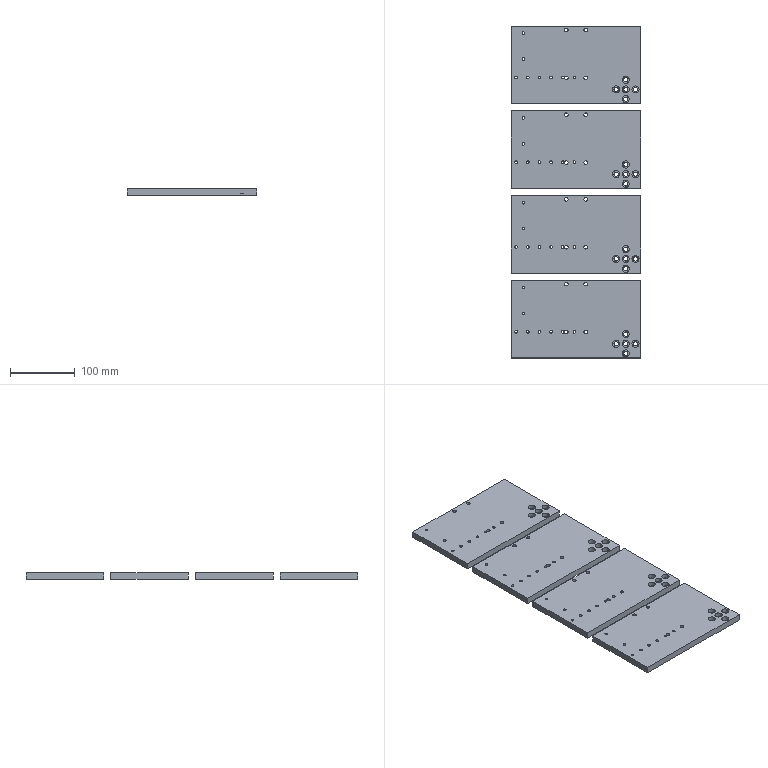Part | 4 solids | 204 faces | box 200 x 513 x 10 mm | volume 927962 mm3 | cylinder 124 | plane 60 | cone 20 | commonest cylinder face diameters 4.134 x52 6.6 x20 11 x20 5.5 x16 10 x16